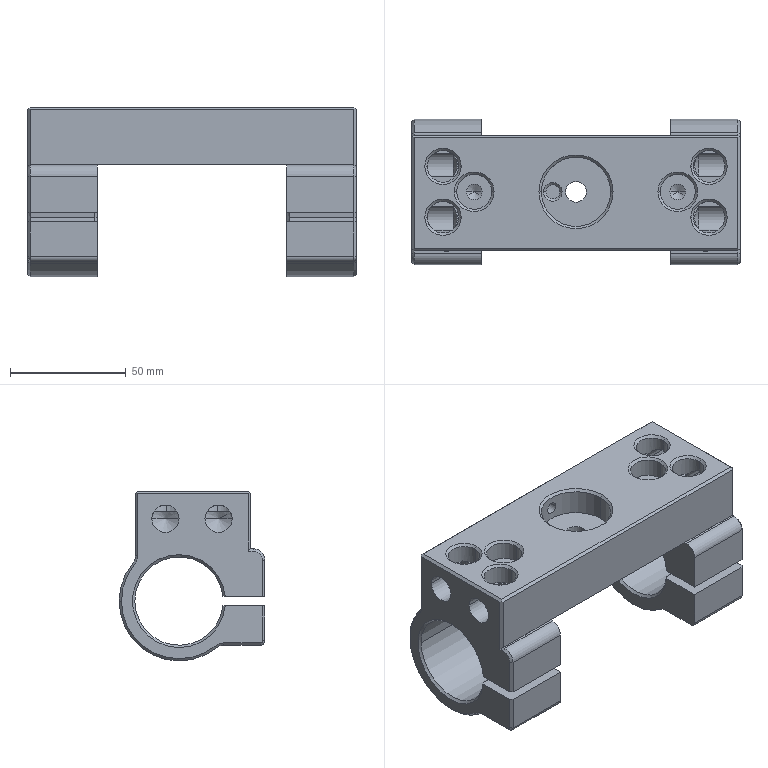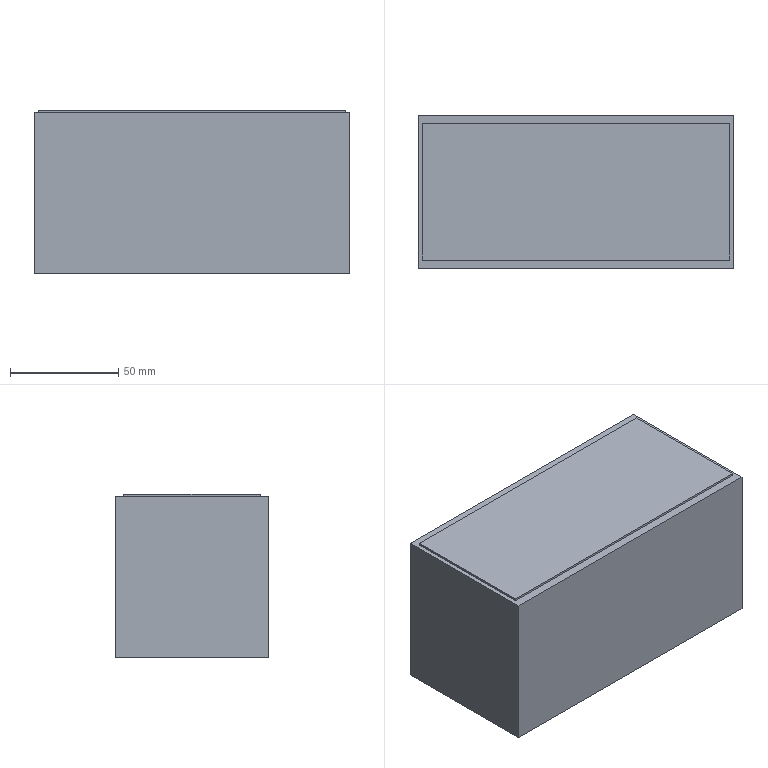CAM job | NX | 3+2 milling, drilling | part box 142 x 63 x 73.5 mm | stock box 146 x 71 x 75.5 mm
Tools:
number,name,description,diameter,corner_radius,flute_length,length,flutes
1,D63,Milling Tool-5 Parameters,63.0,0.0,50.0,75.0,2
7,D6A45,Milling Tool-5 Parameters,6.0,0.0,3.0,3.0,2
16,6.8ZT,Drilling Tool,6.8,0.0,35.0,50.0,2
9,9.0ZT,Drilling Tool,9.0,0.0,35.0,50.0,2
10,D10,Milling Tool-5 Parameters,10.0,0.0,50.0,75.0,2
11,D10JING,Milling Tool-5 Parameters,10.0,0.0,50.0,75.0,2
4,D4,Milling Tool-5 Parameters,4.0,0.0,50.0,75.0,2
2,D100,Milling Tool-5 Parameters,100.0,0.0,50.0,75.0,2
12,11.8ZT,Drilling Tool,11.8,0.0,35.0,50.0,2
8,D8R0.5,Milling Tool-5 Parameters,8.0,0.5,50.0,75.0,2
13,T110H4,Milling Tool-T Cutter,110.0,,4.0,25.0,4
Operations:
program,operation,operation_type,tool,method,geometry_group,spindle_rpm,surface_speed,feed_per_tooth,feed_cut,feed_plunge,cut_length_mm,path_length_mm,cut_time_min,machine_time_min
1-70-75-144毛胚-长度余量单边0.15,FLOOR_WALL,VolumeBased25DMillingOperation,D63,METHOD,A,6500.0,1286.0,0.0962,1250.0,100.0,475.797,529.797,0.3806,0.386
1-70-75-144毛胚-长度余量单边0.15,DRILLING_COPY_1,Operation,D6A45,METHOD,A,3000.0,56.0,0.0333,200.0,0.0,28.0,301.953,0.14,0.1674
1-70-75-144毛胚-长度余量单边0.15,DRILLING_COPY_1_COPY,Operation,6.8ZT,METHOD,A,2000.0,42.0,0.05,200.0,0.0,56.086,263.223,0.2804,0.3011
1-70-75-144毛胚-长度余量单边0.15,DRILLING_COPY_1_COPY_COPY,Operation,9.0ZT,METHOD,A,2000.0,42.0,0.05,200.0,0.0,80.204,394.054,0.401,0.4324
1-70-75-144毛胚-长度余量单边0.15,ADAPTIVE_MILLING,CavityMilling,D10,METHOD,A,8000.0,251.0,0.2188,3500.0,1000.0,12175.462,18393.831,4.151,4.773
1-70-75-144毛胚-长度余量单边0.15,HOLE_MILLING,CylinderMilling,D10,METHOD,A,8000.0,251.0,0.1375,2200.0,100.0,831.709,1409.537,0.378,0.4358
1-70-75-144毛胚-长度余量单边0.15,HOLE_MILLING_COPY,CylinderMilling,D4,METHOD,A,8000.0,100.0,0.0875,1400.0,100.0,131.177,220.677,0.0937,0.1026
1-70-75-144毛胚-长度余量单边0.15,ZLEVEL_PROFILE_COPY_COPY_1,ZLevelMilling,D10JING,METHOD,A,8000.0,251.0,0.05,800.0,100.0,334.118,685.147,0.4176,0.4528
1-70-75-144毛胚-长度余量单边0.15,ZLEVEL_PROFILE_COPY_COPY_1_COPY,ZLevelMilling,D10JING,METHOD,A,8000.0,251.0,0.05,800.0,100.0,334.15,694.221,0.4177,0.4537
1-70-75-144毛胚-长度余量单边0.15,ZLEVEL_PROFILE_COPY_COPY_1_COPY_COPY,ZLevelMilling,D10JING,METHOD,A,8000.0,251.0,0.05,800.0,100.0,268.349,744.827,0.3354,0.3831
1-70-75-144毛胚-长度余量单边0.15,ZLEVEL_PROFILE_COPY_COPY_1_COPY_COPY_COPY,ZLevelMilling,D10JING,METHOD,A,8000.0,251.0,0.05,800.0,100.0,53.918,135.918,0.0674,0.0756
1-70-75-144毛胚-长度余量单边0.15,ZLEVEL_PROFILE_COPY_COPY_1_COPY_COPY_COPY_COPY,ZLevelMilling,D10JING,METHOD,A,8000.0,251.0,0.05,800.0,100.0,68.819,150.819,0.086,0.0942
1-70-75-144毛胚-长度余量单边0.15,ZLEVEL_PROFILE_COPY_COPY_1_COPY_COPY_COPY_COPY_COPY,ZLevelMilling,D10JING,METHOD,A,8000.0,251.0,0.05,800.0,100.0,50.185,291.572,0.0627,0.0869
1-70-75-144毛胚-长度余量单边0.15,ZLEVEL_PROFILE_1_COPY_1_COPY_COPY_1_COPY,ZLevelMilling,D6A45,METHOD,A,7500.0,141.0,0.0667,1000.0,100.0,770.329,1655.643,0.7703,0.8589
1-70-75-144毛胚-长度余量单边0.15,ZLEVEL_PROFILE_1_COPY_1_COPY_COPY_1_COPY_COPY,ZLevelMilling,D6A45,METHOD,A,7500.0,141.0,0.0667,1000.0,100.0,14.697,101.697,0.0147,0.0234
1-70-75-144毛胚-长度余量单边0.15,HOLE_MILLING_COPY_COPY,CylinderMilling,D4,METHOD,A,8000.0,100.0,0.0625,1000.0,100.0,45.828,135.328,0.0458,0.0548
1-70-75-144毛胚-长度余量单边0.15,刀补11,ZLevelMilling,D10JING,METHOD,A,8000.0,251.0,0.05,800.0,100.0,63.713,530.924,0.0796,0.1264
1-70-75-144毛胚-长度余量单边0.15,刀补11.,ZLevelMilling,D10JING,METHOD,A,8000.0,251.0,0.05,800.0,100.0,66.909,148.909,0.0836,0.0918
2-70-75-144毛胚-顶部降0.15对刀,FLOOR_WALL_COPY,VolumeBased25DMillingOperation,D100,METHOD,B,6500.0,1286.0,0.0962,1250.0,100.0,195.5,249.2,0.1564,0.1618
2-70-75-144毛胚-顶部降0.15对刀,FLOOR_WALL_COPY_COPY,VolumeBased25DMillingOperation,D100,METHOD,B,6500.0,1286.0,0.0962,1250.0,100.0,195.5,249.5,0.1564,0.1618
2-70-75-144毛胚-顶部降0.15对刀,DRILLING_COPY_1_COPY_1,Operation,D6A45,METHOD,B,3000.0,56.0,0.0333,200.0,0.0,12.0,152.803,0.06,0.0741
2-70-75-144毛胚-顶部降0.15对刀,DRILLING_COPY_1_COPY_COPY_1,Operation,11.8ZT,METHOD,B,2000.0,42.0,0.05,200.0,0.0,87.135,303.073,0.4357,0.4573
2-70-75-144毛胚-顶部降0.15对刀,HOLE_MILLING_COPY_1,CylinderMilling,D10,METHOD,B,8000.0,251.0,0.1375,2200.0,100.0,2399.138,2488.638,1.091,1.099
2-70-75-144毛胚-顶部降0.15对刀,ZLEVEL_PROFILE_COPY_COPY_1_COPY_1,ZLevelMilling,D10,METHOD,B,8000.0,251.0,0.1562,2500.0,100.0,5186.153,5323.458,2.075,2.088
2-70-75-144毛胚-顶部降0.15对刀,ZLEVEL_PROFILE_COPY_COPY_1_COPY_2,ZLevelMilling,D10JING,METHOD,B,8000.0,251.0,0.05,800.0,100.0,340.893,609.248,0.4261,0.453
2-70-75-144毛胚-顶部降0.15对刀,ZLEVEL_PROFILE_1_COPY_1_COPY_COPY_1_COPY_COPY_1,ZLevelMilling,D6A45,METHOD,B,7500.0,141.0,0.0667,1000.0,100.0,473.58,718.675,0.4736,0.4981
2-70-75-144毛胚-顶部降0.15对刀,刀补11._COPY,ZLevelMilling,D10JING,METHOD,B,8000.0,251.0,0.05,800.0,100.0,185.225,303.334,0.2315,0.2433
3-70-75-144毛胚-顶部降0.15对刀,FLOOR_WALL_COPY_COPY_1,VolumeBased25DMillingOperation,D100,METHOD,C,6500.0,1286.0,0.0962,1250.0,100.0,195.5,249.2,0.1564,0.1618
3-70-75-144毛胚-顶部降0.15对刀,FLOOR_WALL_COPY_COPY_COPY,VolumeBased25DMillingOperation,D100,METHOD,C,6500.0,1286.0,0.0962,1250.0,100.0,195.5,249.5,0.1564,0.1618
3-70-75-144毛胚-顶部降0.15对刀,DRILLING_COPY_1_COPY_1_COPY,Operation,D6A45,METHOD,C,3000.0,56.0,0.0333,200.0,0.0,12.0,149.405,0.06,0.0737
3-70-75-144毛胚-顶部降0.15对刀,DRILLING_COPY_1_COPY_COPY_1_COPY,Operation,11.8ZT,METHOD,C,2000.0,42.0,0.05,200.0,0.0,87.135,299.675,0.4357,0.4569
3-70-75-144毛胚-顶部降0.15对刀,HOLE_MILLING_COPY_1_COPY,CylinderMilling,D10,METHOD,C,8000.0,251.0,0.1375,2200.0,100.0,2399.138,2488.638,1.091,1.099
3-70-75-144毛胚-顶部降0.15对刀,ZLEVEL_PROFILE_COPY_COPY_1_COPY_1_COPY,ZLevelMilling,D10,METHOD,C,8000.0,251.0,0.1562,2500.0,100.0,5201.083,5336.081,2.08,2.094
3-70-75-144毛胚-顶部降0.15对刀,ZLEVEL_PROFILE_COPY_COPY_1_COPY_2_COPY,ZLevelMilling,D10JING,METHOD,C,8000.0,251.0,0.05,800.0,100.0,340.896,609.251,0.4261,0.453
3-70-75-144毛胚-顶部降0.15对刀,ZLEVEL_PROFILE_1_COPY_1_COPY_COPY_1_COPY_COPY_1_COPY,ZLevelMilling,D6A45,METHOD,C,7500.0,141.0,0.0667,1000.0,100.0,473.575,694.119,0.4736,0.4956
3-70-75-144毛胚-顶部降0.15对刀,刀补11._COPY_COPY,ZLevelMilling,D10JING,METHOD,C,8000.0,251.0,0.05,800.0,100.0,185.225,303.334,0.2315,0.2433
4-70-75-144毛胚,DRILLING_COPY_1_COPY_2,Operation,D6A45,METHOD,D,3000.0,56.0,0.0333,200.0,0.0,8.0,191.04,0.04,0.0583
4-70-75-144毛胚,DRILLING_COPY_1_COPY_COPY_2,Operation,6.8ZT,METHOD,D,2000.0,42.0,0.05,200.0,0.0,93.486,362.012,0.4674,0.4943
4-70-75-144毛胚,DRILLING_COPY_1_COPY_COPY_COPY,Operation,9.0ZT,METHOD,D,2000.0,42.0,0.05,200.0,0.0,48.608,272.256,0.243,0.2654
4-70-75-144毛胚,FLOOR_WALL_COPY_1,VolumeBased25DMillingOperation,D63,METHOD,D,5500.0,1088.0,0.2,2200.0,100.0,15840.446,16865.341,7.2,7.303
4-70-75-144毛胚,FLOOR_WALL_COPY_1_COPY,VolumeBased25DMillingOperation,D63,METHOD,D,6500.0,1286.0,0.0923,1200.0,100.0,310.397,453.797,0.2587,0.273
4-70-75-144毛胚,ZLEVEL_PROFILE_COPY_COPY_1_COPY_2_COPY_1,ZLevelMilling,D10JING,METHOD,D,8000.0,251.0,0.05,800.0,100.0,417.625,988.767,0.522,0.5791
4-70-75-144毛胚,HOLE_MILLING_COPY_2,CylinderMilling,D10JING,METHOD,D,8000.0,251.0,0.0938,1500.0,100.0,302.506,553.506,0.2017,0.2268
4-70-75-144毛胚,ZLEVEL_PROFILE_1_COPY_1_COPY_COPY_1_COPY_COPY_1_COPY_COPY,ZLevelMilling,D6A45,METHOD,D,7500.0,141.0,0.0667,1000.0,100.0,118.492,579.182,0.1185,0.1646
4-70-75-144毛胚,ZLEVEL_PROFILE_1_COPY_1_COPY_COPY_1_COPY_COPY_1_COPY_COPY_COPY,ZLevelMilling,D6A45,METHOD,D,7500.0,141.0,0.0667,1000.0,100.0,161.444,502.562,0.1614,0.1956
4-70-75-144毛胚,ZLEVEL_PROFILE_COPY_COPY_1_COPY_2_COPY_1_COPY,ZLevelMilling,D8R0.5,METHOD,D,8000.0,201.0,0.1875,3000.0,1000.0,1480.166,1627.137,0.4953,0.51
4-70-75-144毛胚,PLANAR_MILL,PlanarMilling,T110H4,METHOD,D,4000.0,1382.0,0.0219,350.0,100.0,278.0,374.2,0.7943,0.8039